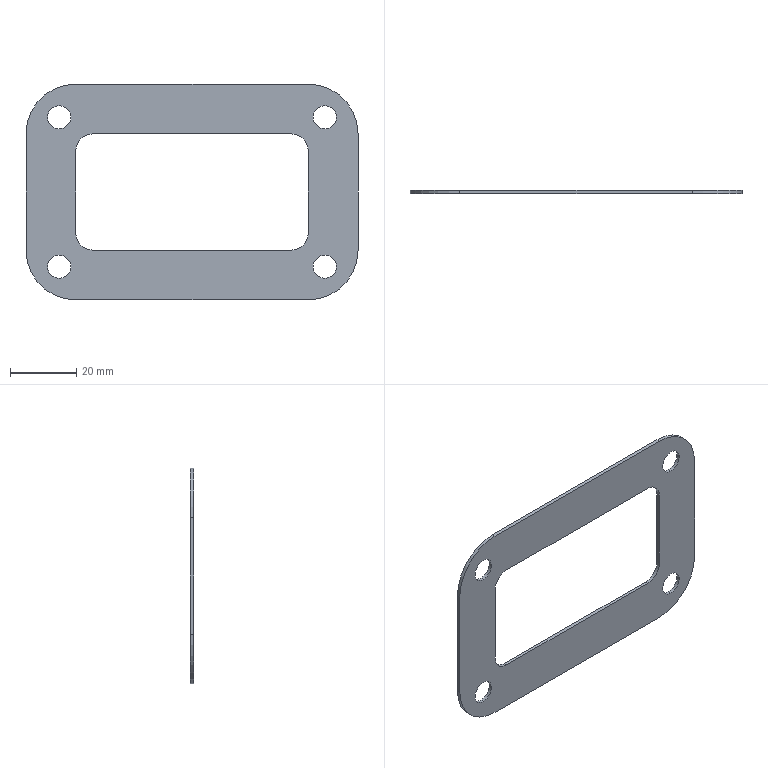Part | SolidWorks | features 3DProfileFeature 1, Extrusion 1, HoleWzd 1, ICE 1, LPattern 1 | 1 solid | 26 faces | box 100 x 1 x 65 mm | volume 3724 mm3 | cylinder 16 | plane 10 | commonest cylinder face diameters 7 x8 10 x4 30 x4
STEP:
#1=CARTESIAN_POINT('',(40.,0.,26.));
#2=VERTEX_POINT('',#1);
#3=CARTESIAN_POINT('',(40.,0.,19.));
#4=VERTEX_POINT('',#3);
#5=CARTESIAN_POINT('',(40.,0.,22.5));
#6=DIRECTION('',(0.,-1.,0.));
#7=DIRECTION('',(0.,0.,-1.));
#8=AXIS2_PLACEMENT_3D('',#5,#6,#7);
#9=CIRCLE('',#8,3.5);
#10=EDGE_CURVE('',#2,#4,#9,.T.);
#11=ORIENTED_EDGE('',*,*,#10,.T.);
#12=CARTESIAN_POINT('',(40.,1.,19.));
#13=VERTEX_POINT('',#12);
#14=CARTESIAN_POINT('',(40.,1.,19.));
#15=DIRECTION('',(0.,1.,0.));
#16=VECTOR('',#15,1000.);
#17=LINE('',#14,#16);
#18=EDGE_CURVE('',#4,#13,#17,.T.);
#19=ORIENTED_EDGE('',*,*,#18,.T.);
#20=CARTESIAN_POINT('',(40.,1.,26.));
#21=VERTEX_POINT('',#20);
#22=CARTESIAN_POINT('',(40.,1.,22.5));
#23=DIRECTION('',(0.,1.,0.));
#24=DIRECTION('',(0.,0.,1.));
#25=AXIS2_PLACEMENT_3D('',#22,#23,#24);
#26=CIRCLE('',#25,3.5);
#27=EDGE_CURVE('',#13,#21,#26,.T.);
#28=ORIENTED_EDGE('',*,*,#27,.T.);
#29=CARTESIAN_POINT('',(40.,1.,26.));
#30=DIRECTION('',(0.,1.,0.));
#31=VECTOR('',#30,1000.);
#32=LINE('',#29,#31);
#33=EDGE_CURVE('',#2,#21,#32,.T.);
#34=ORIENTED_EDGE('',*,*,#33,.F.);
#35=EDGE_LOOP('',(#11,#19,#28,#34));
#36=FACE_OUTER_BOUND('',#35,.T.);
#37=CARTESIAN_POINT('',(40.,1.,22.5));
#38=DIRECTION('',(0.,1.,0.));
#39=DIRECTION('',(0.,0.,1.));
#40=AXIS2_PLACEMENT_3D('',#37,#38,#39);
#41=CYLINDRICAL_SURFACE('',#40,3.5);
#42=ADVANCED_FACE('',(#36),#41,.F.);
#43=CARTESIAN_POINT('',(40.,0.,-19.));
#44=VERTEX_POINT('',#43);
#45=CARTESIAN_POINT('',(40.,0.,-26.));
#46=VERTEX_POINT('',#45);
#47=CARTESIAN_POINT('',(40.,0.,-22.5));
#48=DIRECTION('',(0.,-1.,0.));
#49=DIRECTION('',(0.,0.,-1.));
#50=AXIS2_PLACEMENT_3D('',#47,#48,#49);
#51=CIRCLE('',#50,3.5);
#52=EDGE_CURVE('',#44,#46,#51,.T.);
#53=ORIENTED_EDGE('',*,*,#52,.T.);
#54=CARTESIAN_POINT('',(40.,1.,-26.));
#55=VERTEX_POINT('',#54);
#56=CARTESIAN_POINT('',(40.,1.,-26.));
#57=DIRECTION('',(0.,1.,0.));
#58=VECTOR('',#57,1000.);
#59=LINE('',#56,#58);
#60=EDGE_CURVE('',#46,#55,#59,.T.);
#61=ORIENTED_EDGE('',*,*,#60,.T.);
#62=CARTESIAN_POINT('',(40.,1.,-19.));
#63=VERTEX_POINT('',#62);
#64=CARTESIAN_POINT('',(40.,1.,-22.5));
#65=DIRECTION('',(0.,1.,0.));
#66=DIRECTION('',(0.,0.,1.));
#67=AXIS2_PLACEMENT_3D('',#64,#65,#66);
#68=CIRCLE('',#67,3.5);
#69=EDGE_CURVE('',#55,#63,#68,.T.);
#70=ORIENTED_EDGE('',*,*,#69,.T.);
#71=CARTESIAN_POINT('',(40.,1.,-19.));
#72=DIRECTION('',(0.,1.,0.));
#73=VECTOR('',#72,1000.);
#74=LINE('',#71,#73);
#75=EDGE_CURVE('',#44,#63,#74,.T.);
#76=ORIENTED_EDGE('',*,*,#75,.F.);
#77=EDGE_LOOP('',(#53,#61,#70,#76));
#78=FACE_OUTER_BOUND('',#77,.T.);
#79=CARTESIAN_POINT('',(40.,1.,-22.5));
#80=DIRECTION('',(0.,1.,0.));
#81=DIRECTION('',(0.,0.,1.));
#82=AXIS2_PLACEMENT_3D('',#79,#80,#81);
#83=CYLINDRICAL_SURFACE('',#82,3.5);
#84=ADVANCED_FACE('',(#78),#83,.F.);
#85=CARTESIAN_POINT('',(-40.,0.,26.));
#86=VERTEX_POINT('',#85);
#87=CARTESIAN_POINT('',(-40.,0.,19.));
#88=VERTEX_POINT('',#87);
#89=CARTESIAN_POINT('',(-40.,0.,22.5));
#90=DIRECTION('',(0.,-1.,0.));
#91=DIRECTION('',(0.,0.,-1.));
#92=AXIS2_PLACEMENT_3D('',#89,#90,#91);
#93=CIRCLE('',#92,3.5);
#94=EDGE_CURVE('',#86,#88,#93,.T.);
#95=ORIENTED_EDGE('',*,*,#94,.T.);
#96=CARTESIAN_POINT('',(-40.,1.,19.));
#97=VERTEX_POINT('',#96);
#98=CARTESIAN_POINT('',(-40.,1.,19.));
#99=DIRECTION('',(0.,1.,0.));
#100=VECTOR('',#99,1000.);
#101=LINE('',#98,#100);
#102=EDGE_CURVE('',#88,#97,#101,.T.);
#103=ORIENTED_EDGE('',*,*,#102,.T.);
#104=CARTESIAN_POINT('',(-40.,1.,26.));
#105=VERTEX_POINT('',#104);
#106=CARTESIAN_POINT('',(-40.,1.,22.5));
#107=DIRECTION('',(0.,1.,0.));
#108=DIRECTION('',(0.,0.,1.));
#109=AXIS2_PLACEMENT_3D('',#106,#107,#108);
#110=CIRCLE('',#109,3.5);
#111=EDGE_CURVE('',#97,#105,#110,.T.);
#112=ORIENTED_EDGE('',*,*,#111,.T.);
#113=CARTESIAN_POINT('',(-40.,1.,26.));
#114=DIRECTION('',(0.,1.,0.));
#115=VECTOR('',#114,1000.);
#116=LINE('',#113,#115);
#117=EDGE_CURVE('',#86,#105,#116,.T.);
#118=ORIENTED_EDGE('',*,*,#117,.F.);
#119=EDGE_LOOP('',(#95,#103,#112,#118));
#120=FACE_OUTER_BOUND('',#119,.T.);
#121=CARTESIAN_POINT('',(-40.,1.,22.5));
#122=DIRECTION('',(0.,1.,0.));
#123=DIRECTION('',(0.,0.,1.));
#124=AXIS2_PLACEMENT_3D('',#121,#122,#123);
#125=CYLINDRICAL_SURFACE('',#124,3.5);
#126=ADVANCED_FACE('',(#120),#125,.F.);
#127=CARTESIAN_POINT('',(-40.,0.,-19.));
#128=VERTEX_POINT('',#127);
#129=CARTESIAN_POINT('',(-40.,0.,-26.));
#130=VERTEX_POINT('',#129);
#131=CARTESIAN_POINT('',(-40.,0.,-22.5));
#132=DIRECTION('',(0.,-1.,0.));
#133=DIRECTION('',(0.,0.,-1.));
#134=AXIS2_PLACEMENT_3D('',#131,#132,#133);
#135=CIRCLE('',#134,3.5);
#136=EDGE_CURVE('',#128,#130,#135,.T.);
#137=ORIENTED_EDGE('',*,*,#136,.T.);
#138=CARTESIAN_POINT('',(-40.,1.,-26.));
#139=VERTEX_POINT('',#138);
#140=CARTESIAN_POINT('',(-40.,1.,-26.));
#141=DIRECTION('',(0.,1.,0.));
#142=VECTOR('',#141,1000.);
#143=LINE('',#140,#142);
#144=EDGE_CURVE('',#130,#139,#143,.T.);
#145=ORIENTED_EDGE('',*,*,#144,.T.);
#146=CARTESIAN_POINT('',(-40.,1.,-19.));
#147=VERTEX_POINT('',#146);
#148=CARTESIAN_POINT('',(-40.,1.,-22.5));
#149=DIRECTION('',(0.,1.,0.));
#150=DIRECTION('',(0.,0.,1.));
#151=AXIS2_PLACEMENT_3D('',#148,#149,#150);
#152=CIRCLE('',#151,3.5);
#153=EDGE_CURVE('',#139,#147,#152,.T.);
#154=ORIENTED_EDGE('',*,*,#153,.T.);
#155=CARTESIAN_POINT('',(-40.,1.,-19.));
#156=DIRECTION('',(0.,1.,0.));
#157=VECTOR('',#156,1000.);
#158=LINE('',#155,#157);
#159=EDGE_CURVE('',#128,#147,#158,.T.);
#160=ORIENTED_EDGE('',*,*,#159,.F.);
#161=EDGE_LOOP('',(#137,#145,#154,#160));
#162=FACE_OUTER_BOUND('',#161,.T.);
#163=CARTESIAN_POINT('',(-40.,1.,-22.5));
#164=DIRECTION('',(0.,1.,0.));
#165=DIRECTION('',(0.,0.,1.));
#166=AXIS2_PLACEMENT_3D('',#163,#164,#165);
#167=CYLINDRICAL_SURFACE('',#166,3.5);
#168=ADVANCED_FACE('',(#162),#167,.F.);
#169=CARTESIAN_POINT('',(-40.,1.,22.5));
#170=DIRECTION('',(0.,1.,0.));
#171=DIRECTION('',(0.,0.,1.));
#172=AXIS2_PLACEMENT_3D('',#169,#170,#171);
#173=CIRCLE('',#172,3.5);
#174=EDGE_CURVE('',#105,#97,#173,.T.);
#175=ORIENTED_EDGE('',*,*,#174,.F.);
#176=ORIENTED_EDGE('',*,*,#111,.F.);
#177=EDGE_LOOP('',(#175,#176));
#178=FACE_BOUND('',#177,.T.);
#179=CARTESIAN_POINT('',(-40.,1.,-22.5));
#180=DIRECTION('',(0.,1.,0.));
#181=DIRECTION('',(0.,0.,1.));
#182=AXIS2_PLACEMENT_3D('',#179,#180,#181);
#183=CIRCLE('',#182,3.5);
#184=EDGE_CURVE('',#147,#139,#183,.T.);
#185=ORIENTED_EDGE('',*,*,#184,.F.);
#186=ORIENTED_EDGE('',*,*,#153,.F.);
#187=EDGE_LOOP('',(#185,#186));
#188=FACE_BOUND('',#187,.T.);
#189=CARTESIAN_POINT('',(30.,1.,-17.5));
#190=VERTEX_POINT('',#189);
#191=CARTESIAN_POINT('',(-30.,1.,-17.5));
#192=VERTEX_POINT('',#191);
#193=CARTESIAN_POINT('',(-30.,1.,-17.5));
#194=DIRECTION('',(-1.,0.,0.));
#195=VECTOR('',#194,1000.);
#196=LINE('',#193,#195);
#197=EDGE_CURVE('',#190,#192,#196,.T.);
#198=ORIENTED_EDGE('',*,*,#197,.F.);
#199=CARTESIAN_POINT('',(35.,1.,-12.5));
#200=VERTEX_POINT('',#199);
#201=CARTESIAN_POINT('',(30.,1.,-12.5));
#202=DIRECTION('',(0.,1.,0.));
#203=DIRECTION('',(0.,0.,-1.));
#204=AXIS2_PLACEMENT_3D('',#201,#202,#203);
#205=CIRCLE('',#204,5.);
#206=EDGE_CURVE('',#200,#190,#205,.T.);
#207=ORIENTED_EDGE('',*,*,#206,.F.);
#208=CARTESIAN_POINT('',(35.,1.,12.5));
#209=VERTEX_POINT('',#208);
#210=CARTESIAN_POINT('',(35.,1.,-12.5));
#211=DIRECTION('',(0.,0.,-1.));
#212=VECTOR('',#211,1000.);
#213=LINE('',#210,#212);
#214=EDGE_CURVE('',#209,#200,#213,.T.);
#215=ORIENTED_EDGE('',*,*,#214,.F.);
#216=CARTESIAN_POINT('',(30.,1.,17.5));
#217=VERTEX_POINT('',#216);
#218=CARTESIAN_POINT('',(30.,1.,12.5));
#219=DIRECTION('',(0.,1.,0.));
#220=DIRECTION('',(0.,0.,1.));
#221=AXIS2_PLACEMENT_3D('',#218,#219,#220);
#222=CIRCLE('',#221,5.);
#223=EDGE_CURVE('',#217,#209,#222,.T.);
#224=ORIENTED_EDGE('',*,*,#223,.F.);
#225=CARTESIAN_POINT('',(-30.,1.,17.5));
#226=VERTEX_POINT('',#225);
#227=CARTESIAN_POINT('',(-30.,1.,17.5));
#228=DIRECTION('',(1.,0.,0.));
#229=VECTOR('',#228,1000.);
#230=LINE('',#227,#229);
#231=EDGE_CURVE('',#226,#217,#230,.T.);
#232=ORIENTED_EDGE('',*,*,#231,.F.);
#233=CARTESIAN_POINT('',(-35.,1.,12.5));
#234=VERTEX_POINT('',#233);
#235=CARTESIAN_POINT('',(-30.,1.,12.5));
#236=DIRECTION('',(0.,1.,0.));
#237=DIRECTION('',(0.,0.,1.));
#238=AXIS2_PLACEMENT_3D('',#235,#236,#237);
#239=CIRCLE('',#238,5.);
#240=EDGE_CURVE('',#234,#226,#239,.T.);
#241=ORIENTED_EDGE('',*,*,#240,.F.);
#242=CARTESIAN_POINT('',(-35.,1.,-12.5));
#243=VERTEX_POINT('',#242);
#244=CARTESIAN_POINT('',(-35.,1.,-12.5));
#245=DIRECTION('',(0.,0.,1.));
#246=VECTOR('',#245,1000.);
#247=LINE('',#244,#246);
#248=EDGE_CURVE('',#243,#234,#247,.T.);
#249=ORIENTED_EDGE('',*,*,#248,.F.);
#250=CARTESIAN_POINT('',(-30.,1.,-12.5));
#251=DIRECTION('',(0.,1.,0.));
#252=DIRECTION('',(0.,0.,1.));
#253=AXIS2_PLACEMENT_3D('',#250,#251,#252);
#254=CIRCLE('',#253,5.);
#255=EDGE_CURVE('',#192,#243,#254,.T.);
#256=ORIENTED_EDGE('',*,*,#255,.F.);
#257=EDGE_LOOP('',(#198,#207,#215,#224,#232,#241,#249,#256));
#258=FACE_BOUND('',#257,.T.);
#259=CARTESIAN_POINT('',(50.,1.,-17.5));
#260=VERTEX_POINT('',#259);
#261=CARTESIAN_POINT('',(35.,1.,-32.5));
#262=VERTEX_POINT('',#261);
#263=CARTESIAN_POINT('',(35.,1.,-17.5));
#264=DIRECTION('',(0.,1.,0.));
#265=DIRECTION('',(0.,0.,-1.));
#266=AXIS2_PLACEMENT_3D('',#263,#264,#265);
#267=CIRCLE('',#266,15.);
#268=EDGE_CURVE('',#260,#262,#267,.T.);
#269=ORIENTED_EDGE('',*,*,#268,.T.);
#270=CARTESIAN_POINT('',(-35.,1.,-32.5));
#271=VERTEX_POINT('',#270);
#272=CARTESIAN_POINT('',(-35.,1.,-32.5));
#273=DIRECTION('',(-1.,0.,0.));
#274=VECTOR('',#273,1000.);
#275=LINE('',#272,#274);
#276=EDGE_CURVE('',#262,#271,#275,.T.);
#277=ORIENTED_EDGE('',*,*,#276,.T.);
#278=CARTESIAN_POINT('',(-50.,1.,-17.5));
#279=VERTEX_POINT('',#278);
#280=CARTESIAN_POINT('',(-35.,1.,-17.5));
#281=DIRECTION('',(0.,1.,0.));
#282=DIRECTION('',(0.,0.,1.));
#283=AXIS2_PLACEMENT_3D('',#280,#281,#282);
#284=CIRCLE('',#283,15.);
#285=EDGE_CURVE('',#271,#279,#284,.T.);
#286=ORIENTED_EDGE('',*,*,#285,.T.);
#287=CARTESIAN_POINT('',(-50.,1.,17.5));
#288=VERTEX_POINT('',#287);
#289=CARTESIAN_POINT('',(-50.,1.,-17.5));
#290=DIRECTION('',(0.,0.,1.));
#291=VECTOR('',#290,1000.);
#292=LINE('',#289,#291);
#293=EDGE_CURVE('',#279,#288,#292,.T.);
#294=ORIENTED_EDGE('',*,*,#293,.T.);
#295=CARTESIAN_POINT('',(-35.,1.,32.5));
#296=VERTEX_POINT('',#295);
#297=CARTESIAN_POINT('',(-35.,1.,17.5));
#298=DIRECTION('',(0.,1.,0.));
#299=DIRECTION('',(0.,0.,1.));
#300=AXIS2_PLACEMENT_3D('',#297,#298,#299);
#301=CIRCLE('',#300,15.);
#302=EDGE_CURVE('',#288,#296,#301,.T.);
#303=ORIENTED_EDGE('',*,*,#302,.T.);
#304=CARTESIAN_POINT('',(35.,1.,32.5));
#305=VERTEX_POINT('',#304);
#306=CARTESIAN_POINT('',(-35.,1.,32.5));
#307=DIRECTION('',(1.,0.,0.));
#308=VECTOR('',#307,1000.);
#309=LINE('',#306,#308);
#310=EDGE_CURVE('',#296,#305,#309,.T.);
#311=ORIENTED_EDGE('',*,*,#310,.T.);
#312=CARTESIAN_POINT('',(50.,1.,17.5));
#313=VERTEX_POINT('',#312);
#314=CARTESIAN_POINT('',(35.,1.,17.5));
#315=DIRECTION('',(0.,1.,0.));
#316=DIRECTION('',(0.,0.,1.));
#317=AXIS2_PLACEMENT_3D('',#314,#315,#316);
#318=CIRCLE('',#317,15.);
#319=EDGE_CURVE('',#305,#313,#318,.T.);
#320=ORIENTED_EDGE('',*,*,#319,.T.);
#321=CARTESIAN_POINT('',(50.,1.,-17.5));
#322=DIRECTION('',(0.,0.,-1.));
#323=VECTOR('',#322,1000.);
#324=LINE('',#321,#323);
#325=EDGE_CURVE('',#313,#260,#324,.T.);
#326=ORIENTED_EDGE('',*,*,#325,.T.);
#327=EDGE_LOOP('',(#269,#277,#286,#294,#303,#311,#320,#326));
#328=FACE_OUTER_BOUND('',#327,.T.);
#329=CARTESIAN_POINT('',(40.,1.,-22.5));
#330=DIRECTION('',(0.,1.,0.));
#331=DIRECTION('',(0.,0.,1.));
#332=AXIS2_PLACEMENT_3D('',#329,#330,#331);
#333=CIRCLE('',#332,3.5);
#334=EDGE_CURVE('',#63,#55,#333,.T.);
#335=ORIENTED_EDGE('',*,*,#334,.F.);
#336=ORIENTED_EDGE('',*,*,#69,.F.);
#337=EDGE_LOOP('',(#335,#336));
#338=FACE_BOUND('',#337,.T.);
#339=CARTESIAN_POINT('',(40.,1.,22.5));
#340=DIRECTION('',(0.,1.,0.));
#341=DIRECTION('',(0.,0.,1.));
#342=AXIS2_PLACEMENT_3D('',#339,#340,#341);
#343=CIRCLE('',#342,3.5);
#344=EDGE_CURVE('',#21,#13,#343,.T.);
#345=ORIENTED_EDGE('',*,*,#344,.F.);
#346=ORIENTED_EDGE('',*,*,#27,.F.);
#347=EDGE_LOOP('',(#345,#346));
#348=FACE_BOUND('',#347,.T.);
#349=CARTESIAN_POINT('',(35.,1.,-17.5));
#350=DIRECTION('',(0.,-1.,0.));
#351=DIRECTION('',(0.,0.,-1.));
#352=AXIS2_PLACEMENT_3D('',#349,#350,#351);
#353=PLANE('',#352);
#354=ADVANCED_FACE('',(#178,#188,#258,#328,#338,#348),#353,.F.);
#355=CARTESIAN_POINT('',(50.,0.,-17.5));
#356=VERTEX_POINT('',#355);
#357=CARTESIAN_POINT('',(35.,0.,-32.5));
#358=VERTEX_POINT('',#357);
#359=CARTESIAN_POINT('',(35.,0.,-17.5));
#360=DIRECTION('',(0.,1.,0.));
#361=DIRECTION('',(0.,0.,-1.));
#362=AXIS2_PLACEMENT_3D('',#359,#360,#361);
#363=CIRCLE('',#362,15.);
#364=EDGE_CURVE('',#356,#358,#363,.T.);
#365=ORIENTED_EDGE('',*,*,#364,.T.);
#366=CARTESIAN_POINT('',(35.,1.,-32.5));
#367=DIRECTION('',(0.,-1.,0.));
#368=VECTOR('',#367,1000.);
#369=LINE('',#366,#368);
#370=EDGE_CURVE('',#262,#358,#369,.T.);
#371=ORIENTED_EDGE('',*,*,#370,.F.);
#372=ORIENTED_EDGE('',*,*,#268,.F.);
#373=CARTESIAN_POINT('',(50.,1.,-17.5));
#374=DIRECTION('',(0.,-1.,0.));
#375=VECTOR('',#374,1000.);
#376=LINE('',#373,#375);
#377=EDGE_CURVE('',#260,#356,#376,.T.);
#378=ORIENTED_EDGE('',*,*,#377,.T.);
#379=EDGE_LOOP('',(#365,#371,#372,#378));
#380=FACE_OUTER_BOUND('',#379,.T.);
#381=CARTESIAN_POINT('',(35.,1.,-17.5));
#382=DIRECTION('',(0.,-1.,0.));
#383=DIRECTION('',(0.,0.,-1.));
#384=AXIS2_PLACEMENT_3D('',#381,#382,#383);
#385=CYLINDRICAL_SURFACE('',#384,15.);
#386=ADVANCED_FACE('',(#380),#385,.T.);
#387=CARTESIAN_POINT('',(-35.,0.,-32.5));
#388=VERTEX_POINT('',#387);
#389=CARTESIAN_POINT('',(-35.,0.,-32.5));
#390=DIRECTION('',(-1.,0.,0.));
#391=VECTOR('',#390,1000.);
#392=LINE('',#389,#391);
#393=EDGE_CURVE('',#358,#388,#392,.T.);
#394=ORIENTED_EDGE('',*,*,#393,.T.);
#395=CARTESIAN_POINT('',(-35.,1.,-32.5));
#396=DIRECTION('',(0.,-1.,0.));
#397=VECTOR('',#396,1000.);
#398=LINE('',#395,#397);
#399=EDGE_CURVE('',#271,#388,#398,.T.);
#400=ORIENTED_EDGE('',*,*,#399,.F.);
#401=ORIENTED_EDGE('',*,*,#276,.F.);
#402=ORIENTED_EDGE('',*,*,#370,.T.);
#403=EDGE_LOOP('',(#394,#400,#401,#402));
#404=FACE_OUTER_BOUND('',#403,.T.);
#405=CARTESIAN_POINT('',(-35.,1.,-32.5));
#406=DIRECTION('',(0.,0.,1.));
#407=DIRECTION('',(1.,0.,0.));
#408=AXIS2_PLACEMENT_3D('',#405,#406,#407);
#409=PLANE('',#408);
#410=ADVANCED_FACE('',(#404),#409,.F.);
#411=CARTESIAN_POINT('',(-50.,0.,-17.5));
#412=VERTEX_POINT('',#411);
#413=CARTESIAN_POINT('',(-35.,0.,-17.5));
#414=DIRECTION('',(0.,1.,0.));
#415=DIRECTION('',(0.,0.,1.));
#416=AXIS2_PLACEMENT_3D('',#413,#414,#415);
#417=CIRCLE('',#416,15.);
#418=EDGE_CURVE('',#388,#412,#417,.T.);
#419=ORIENTED_EDGE('',*,*,#418,.T.);
#420=CARTESIAN_POINT('',(-50.,1.,-17.5));
#421=DIRECTION('',(0.,-1.,0.));
#422=VECTOR('',#421,1000.);
#423=LINE('',#420,#422);
#424=EDGE_CURVE('',#279,#412,#423,.T.);
#425=ORIENTED_EDGE('',*,*,#424,.F.);
#426=ORIENTED_EDGE('',*,*,#285,.F.);
#427=ORIENTED_EDGE('',*,*,#399,.T.);
#428=EDGE_LOOP('',(#419,#425,#426,#427));
#429=FACE_OUTER_BOUND('',#428,.T.);
#430=CARTESIAN_POINT('',(-35.,1.,-17.5));
#431=DIRECTION('',(0.,-1.,0.));
#432=DIRECTION('',(0.,0.,-1.));
#433=AXIS2_PLACEMENT_3D('',#430,#431,#432);
#434=CYLINDRICAL_SURFACE('',#433,15.);
#435=ADVANCED_FACE('',(#429),#434,.T.);
#436=CARTESIAN_POINT('',(-50.,0.,17.5));
#437=VERTEX_POINT('',#436);
#438=CARTESIAN_POINT('',(-50.,0.,-17.5));
#439=DIRECTION('',(0.,0.,1.));
#440=VECTOR('',#439,1000.);
#441=LINE('',#438,#440);
#442=EDGE_CURVE('',#412,#437,#441,.T.);
#443=ORIENTED_EDGE('',*,*,#442,.T.);
#444=CARTESIAN_POINT('',(-50.,1.,17.5));
#445=DIRECTION('',(0.,-1.,0.));
#446=VECTOR('',#445,1000.);
#447=LINE('',#444,#446);
#448=EDGE_CURVE('',#288,#437,#447,.T.);
#449=ORIENTED_EDGE('',*,*,#448,.F.);
#450=ORIENTED_EDGE('',*,*,#293,.F.);
#451=ORIENTED_EDGE('',*,*,#424,.T.);
#452=EDGE_LOOP('',(#443,#449,#450,#451));
#453=FACE_OUTER_BOUND('',#452,.T.);
#454=CARTESIAN_POINT('',(-50.,1.,-17.5));
#455=DIRECTION('',(1.,0.,0.));
#456=DIRECTION('',(0.,0.,-1.));
#457=AXIS2_PLACEMENT_3D('',#454,#455,#456);
#458=PLANE('',#457);
#459=ADVANCED_FACE('',(#453),#458,.F.);
#460=CARTESIAN_POINT('',(-35.,0.,32.5));
#461=VERTEX_POINT('',#460);
#462=CARTESIAN_POINT('',(-35.,0.,17.5));
#463=DIRECTION('',(0.,1.,0.));
#464=DIRECTION('',(0.,0.,1.));
#465=AXIS2_PLACEMENT_3D('',#462,#463,#464);
#466=CIRCLE('',#465,15.);
#467=EDGE_CURVE('',#437,#461,#466,.T.);
#468=ORIENTED_EDGE('',*,*,#467,.T.);
#469=CARTESIAN_POINT('',(-35.,1.,32.5));
#470=DIRECTION('',(0.,-1.,0.));
#471=VECTOR('',#470,1000.);
#472=LINE('',#469,#471);
#473=EDGE_CURVE('',#296,#461,#472,.T.);
#474=ORIENTED_EDGE('',*,*,#473,.F.);
#475=ORIENTED_EDGE('',*,*,#302,.F.);
#476=ORIENTED_EDGE('',*,*,#448,.T.);
#477=EDGE_LOOP('',(#468,#474,#475,#476));
#478=FACE_OUTER_BOUND('',#477,.T.);
#479=CARTESIAN_POINT('',(-35.,1.,17.5));
#480=DIRECTION('',(0.,-1.,0.));
#481=DIRECTION('',(0.,0.,-1.));
#482=AXIS2_PLACEMENT_3D('',#479,#480,#481);
#483=CYLINDRICAL_SURFACE('',#482,15.);
#484=ADVANCED_FACE('',(#478),#483,.T.);
#485=CARTESIAN_POINT('',(35.,0.,32.5));
#486=VERTEX_POINT('',#485);
#487=CARTESIAN_POINT('',(-35.,0.,32.5));
#488=DIRECTION('',(1.,0.,0.));
#489=VECTOR('',#488,1000.);
#490=LINE('',#487,#489);
#491=EDGE_CURVE('',#461,#486,#490,.T.);
#492=ORIENTED_EDGE('',*,*,#491,.T.);
#493=CARTESIAN_POINT('',(35.,1.,32.5));
#494=DIRECTION('',(0.,-1.,0.));
#495=VECTOR('',#494,1000.);
#496=LINE('',#493,#495);
#497=EDGE_CURVE('',#305,#486,#496,.T.);
#498=ORIENTED_EDGE('',*,*,#497,.F.);
#499=ORIENTED_EDGE('',*,*,#310,.F.);
#500=ORIENTED_EDGE('',*,*,#473,.T.);
#501=EDGE_LOOP('',(#492,#498,#499,#500));
#502=FACE_OUTER_BOUND('',#501,.T.);
#503=CARTESIAN_POINT('',(-35.,1.,32.5));
#504=DIRECTION('',(0.,0.,-1.));
#505=DIRECTION('',(-1.,0.,0.));
#506=AXIS2_PLACEMENT_3D('',#503,#504,#505);
#507=PLANE('',#506);
#508=ADVANCED_FACE('',(#502),#507,.F.);
#509=CARTESIAN_POINT('',(50.,0.,17.5));
#510=VERTEX_POINT('',#509);
#511=CARTESIAN_POINT('',(35.,0.,17.5));
#512=DIRECTION('',(0.,1.,0.));
#513=DIRECTION('',(0.,0.,1.));
#514=AXIS2_PLACEMENT_3D('',#511,#512,#513);
#515=CIRCLE('',#514,15.);
#516=EDGE_CURVE('',#486,#510,#515,.T.);
#517=ORIENTED_EDGE('',*,*,#516,.T.);
#518=CARTESIAN_POINT('',(50.,1.,17.5));
#519=DIRECTION('',(0.,-1.,0.));
#520=VECTOR('',#519,1000.);
#521=LINE('',#518,#520);
#522=EDGE_CURVE('',#313,#510,#521,.T.);
#523=ORIENTED_EDGE('',*,*,#522,.F.);
#524=ORIENTED_EDGE('',*,*,#319,.F.);
#525=ORIENTED_EDGE('',*,*,#497,.T.);
#526=EDGE_LOOP('',(#517,#523,#524,#525));
#527=FACE_OUTER_BOUND('',#526,.T.);
#528=CARTESIAN_POINT('',(35.,1.,17.5));
#529=DIRECTION('',(0.,-1.,0.));
#530=DIRECTION('',(0.,0.,-1.));
#531=AXIS2_PLACEMENT_3D('',#528,#529,#530);
#532=CYLINDRICAL_SURFACE('',#531,15.);
#533=ADVANCED_FACE('',(#527),#532,.T.);
#534=CARTESIAN_POINT('',(50.,0.,-17.5));
#535=DIRECTION('',(0.,0.,-1.));
#536=VECTOR('',#535,1000.);
#537=LINE('',#534,#536);
#538=EDGE_CURVE('',#510,#356,#537,.T.);
#539=ORIENTED_EDGE('',*,*,#538,.T.);
#540=ORIENTED_EDGE('',*,*,#377,.F.);
#541=ORIENTED_EDGE('',*,*,#325,.F.);
#542=ORIENTED_EDGE('',*,*,#522,.T.);
#543=EDGE_LOOP('',(#539,#540,#541,#542));
#544=FACE_OUTER_BOUND('',#543,.T.);
#545=CARTESIAN_POINT('',(50.,1.,-17.5));
#546=DIRECTION('',(-1.,0.,0.));
#547=DIRECTION('',(0.,0.,1.));
#548=AXIS2_PLACEMENT_3D('',#545,#546,#547);
#549=PLANE('',#548);
#550=ADVANCED_FACE('',(#544),#549,.F.);
#551=ORIENTED_EDGE('',*,*,#10,.F.);
#552=CARTESIAN_POINT('',(40.,0.,22.5));
#553=DIRECTION('',(0.,-1.,0.));
#554=DIRECTION('',(0.,0.,-1.));
#555=AXIS2_PLACEMENT_3D('',#552,#553,#554);
#556=CIRCLE('',#555,3.5);
#557=EDGE_CURVE('',#4,#2,#556,.T.);
#558=ORIENTED_EDGE('',*,*,#557,.F.);
#559=EDGE_LOOP('',(#551,#558));
#560=FACE_BOUND('',#559,.T.);
#561=ORIENTED_EDGE('',*,*,#52,.F.);
#562=CARTESIAN_POINT('',(40.,0.,-22.5));
#563=DIRECTION('',(0.,-1.,0.));
#564=DIRECTION('',(0.,0.,-1.));
#565=AXIS2_PLACEMENT_3D('',#562,#563,#564);
#566=CIRCLE('',#565,3.5);
#567=EDGE_CURVE('',#46,#44,#566,.T.);
#568=ORIENTED_EDGE('',*,*,#567,.F.);
#569=EDGE_LOOP('',(#561,#568));
#570=FACE_BOUND('',#569,.T.);
#571=ORIENTED_EDGE('',*,*,#94,.F.);
#572=CARTESIAN_POINT('',(-40.,0.,22.5));
#573=DIRECTION('',(0.,-1.,0.));
#574=DIRECTION('',(0.,0.,-1.));
#575=AXIS2_PLACEMENT_3D('',#572,#573,#574);
#576=CIRCLE('',#575,3.5);
#577=EDGE_CURVE('',#88,#86,#576,.T.);
#578=ORIENTED_EDGE('',*,*,#577,.F.);
#579=EDGE_LOOP('',(#571,#578));
#580=FACE_BOUND('',#579,.T.);
#581=ORIENTED_EDGE('',*,*,#136,.F.);
#582=CARTESIAN_POINT('',(-40.,0.,-22.5));
#583=DIRECTION('',(0.,-1.,0.));
#584=DIRECTION('',(0.,0.,-1.));
#585=AXIS2_PLACEMENT_3D('',#582,#583,#584);
#586=CIRCLE('',#585,3.5);
#587=EDGE_CURVE('',#130,#128,#586,.T.);
#588=ORIENTED_EDGE('',*,*,#587,.F.);
#589=EDGE_LOOP('',(#581,#588));
#590=FACE_BOUND('',#589,.T.);
#591=CARTESIAN_POINT('',(35.,0.,-12.5));
#592=VERTEX_POINT('',#591);
#593=CARTESIAN_POINT('',(30.,0.,-17.5));
#594=VERTEX_POINT('',#593);
#595=CARTESIAN_POINT('',(30.,0.,-12.5));
#596=DIRECTION('',(0.,1.,0.));
#597=DIRECTION('',(0.,0.,-1.));
#598=AXIS2_PLACEMENT_3D('',#595,#596,#597);
#599=CIRCLE('',#598,5.);
#600=EDGE_CURVE('',#592,#594,#599,.T.);
#601=ORIENTED_EDGE('',*,*,#600,.T.);
#602=CARTESIAN_POINT('',(-30.,0.,-17.5));
#603=VERTEX_POINT('',#602);
#604=CARTESIAN_POINT('',(-30.,0.,-17.5));
#605=DIRECTION('',(-1.,0.,0.));
#606=VECTOR('',#605,1000.);
#607=LINE('',#604,#606);
#608=EDGE_CURVE('',#594,#603,#607,.T.);
#609=ORIENTED_EDGE('',*,*,#608,.T.);
#610=CARTESIAN_POINT('',(-35.,0.,-12.5));
#611=VERTEX_POINT('',#610);
#612=CARTESIAN_POINT('',(-30.,0.,-12.5));
#613=DIRECTION('',(0.,1.,0.));
#614=DIRECTION('',(0.,0.,1.));
#615=AXIS2_PLACEMENT_3D('',#612,#613,#614);
#616=CIRCLE('',#615,5.);
#617=EDGE_CURVE('',#603,#611,#616,.T.);
#618=ORIENTED_EDGE('',*,*,#617,.T.);
#619=CARTESIAN_POINT('',(-35.,0.,12.5));
#620=VERTEX_POINT('',#619);
#621=CARTESIAN_POINT('',(-35.,0.,-12.5));
#622=DIRECTION('',(0.,0.,1.));
#623=VECTOR('',#622,1000.);
#624=LINE('',#621,#623);
#625=EDGE_CURVE('',#611,#620,#624,.T.);
#626=ORIENTED_EDGE('',*,*,#625,.T.);
#627=CARTESIAN_POINT('',(-30.,0.,17.5));
#628=VERTEX_POINT('',#627);
#629=CARTESIAN_POINT('',(-30.,0.,12.5));
#630=DIRECTION('',(0.,1.,0.));
#631=DIRECTION('',(0.,0.,1.));
#632=AXIS2_PLACEMENT_3D('',#629,#630,#631);
#633=CIRCLE('',#632,5.);
#634=EDGE_CURVE('',#620,#628,#633,.T.);
#635=ORIENTED_EDGE('',*,*,#634,.T.);
#636=CARTESIAN_POINT('',(30.,0.,17.5));
#637=VERTEX_POINT('',#636);
#638=CARTESIAN_POINT('',(-30.,0.,17.5));
#639=DIRECTION('',(1.,0.,0.));
#640=VECTOR('',#639,1000.);
#641=LINE('',#638,#640);
#642=EDGE_CURVE('',#628,#637,#641,.T.);
#643=ORIENTED_EDGE('',*,*,#642,.T.);
#644=CARTESIAN_POINT('',(35.,0.,12.5));
#645=VERTEX_POINT('',#644);
#646=CARTESIAN_POINT('',(30.,0.,12.5));
#647=DIRECTION('',(0.,1.,0.));
#648=DIRECTION('',(0.,0.,1.));
#649=AXIS2_PLACEMENT_3D('',#646,#647,#648);
#650=CIRCLE('',#649,5.);
#651=EDGE_CURVE('',#637,#645,#650,.T.);
#652=ORIENTED_EDGE('',*,*,#651,.T.);
#653=CARTESIAN_POINT('',(35.,0.,-12.5));
#654=DIRECTION('',(0.,0.,-1.));
#655=VECTOR('',#654,1000.);
#656=LINE('',#653,#655);
#657=EDGE_CURVE('',#645,#592,#656,.T.);
#658=ORIENTED_EDGE('',*,*,#657,.T.);
#659=EDGE_LOOP('',(#601,#609,#618,#626,#635,#643,#652,#658));
#660=FACE_BOUND('',#659,.T.);
#661=ORIENTED_EDGE('',*,*,#364,.F.);
#662=ORIENTED_EDGE('',*,*,#538,.F.);
#663=ORIENTED_EDGE('',*,*,#516,.F.);
#664=ORIENTED_EDGE('',*,*,#491,.F.);
#665=ORIENTED_EDGE('',*,*,#467,.F.);
#666=ORIENTED_EDGE('',*,*,#442,.F.);
#667=ORIENTED_EDGE('',*,*,#418,.F.);
#668=ORIENTED_EDGE('',*,*,#393,.F.);
#669=EDGE_LOOP('',(#661,#662,#663,#664,#665,#666,#667,#668));
#670=FACE_OUTER_BOUND('',#669,.T.);
#671=CARTESIAN_POINT('',(35.,0.,-17.5));
#672=DIRECTION('',(0.,-1.,0.));
#673=DIRECTION('',(0.,0.,-1.));
#674=AXIS2_PLACEMENT_3D('',#671,#672,#673);
#675=PLANE('',#674);
#676=ADVANCED_FACE('',(#560,#570,#580,#590,#660,#670),#675,.T.);
#677=ORIENTED_EDGE('',*,*,#206,.T.);
#678=CARTESIAN_POINT('',(30.,0.,-17.5));
#679=DIRECTION('',(0.,1.,0.));
#680=VECTOR('',#679,1000.);
#681=LINE('',#678,#680);
#682=EDGE_CURVE('',#594,#190,#681,.T.);
#683=ORIENTED_EDGE('',*,*,#682,.F.);
#684=ORIENTED_EDGE('',*,*,#600,.F.);
#685=CARTESIAN_POINT('',(35.,0.,-12.5));
#686=DIRECTION('',(0.,1.,0.));
#687=VECTOR('',#686,1000.);
#688=LINE('',#685,#687);
#689=EDGE_CURVE('',#592,#200,#688,.T.);
#690=ORIENTED_EDGE('',*,*,#689,.T.);
#691=EDGE_LOOP('',(#677,#683,#684,#690));
#692=FACE_OUTER_BOUND('',#691,.T.);
#693=CARTESIAN_POINT('',(30.,0.,-12.5));
#694=DIRECTION('',(0.,1.,0.));
#695=DIRECTION('',(0.,0.,1.));
#696=AXIS2_PLACEMENT_3D('',#693,#694,#695);
#697=CYLINDRICAL_SURFACE('',#696,5.);
#698=ADVANCED_FACE('',(#692),#697,.F.);
#699=ORIENTED_EDGE('',*,*,#214,.T.);
#700=ORIENTED_EDGE('',*,*,#689,.F.);
#701=ORIENTED_EDGE('',*,*,#657,.F.);
#702=CARTESIAN_POINT('',(35.,0.,12.5));
#703=DIRECTION('',(0.,1.,0.));
#704=VECTOR('',#703,1000.);
#705=LINE('',#702,#704);
#706=EDGE_CURVE('',#645,#209,#705,.T.);
#707=ORIENTED_EDGE('',*,*,#706,.T.);
#708=EDGE_LOOP('',(#699,#700,#701,#707));
#709=FACE_OUTER_BOUND('',#708,.T.);
#710=CARTESIAN_POINT('',(35.,0.,-12.5));
#711=DIRECTION('',(1.,0.,0.));
#712=DIRECTION('',(0.,0.,-1.));
#713=AXIS2_PLACEMENT_3D('',#710,#711,#712);
#714=PLANE('',#713);
#715=ADVANCED_FACE('',(#709),#714,.F.);
#716=ORIENTED_EDGE('',*,*,#223,.T.);
#717=ORIENTED_EDGE('',*,*,#706,.F.);
#718=ORIENTED_EDGE('',*,*,#651,.F.);
#719=CARTESIAN_POINT('',(30.,0.,17.5));
#720=DIRECTION('',(0.,1.,0.));
#721=VECTOR('',#720,1000.);
#722=LINE('',#719,#721);
#723=EDGE_CURVE('',#637,#217,#722,.T.);
#724=ORIENTED_EDGE('',*,*,#723,.T.);
#725=EDGE_LOOP('',(#716,#717,#718,#724));
#726=FACE_OUTER_BOUND('',#725,.T.);
#727=CARTESIAN_POINT('',(30.,0.,12.5));
#728=DIRECTION('',(0.,1.,0.));
#729=DIRECTION('',(0.,0.,1.));
#730=AXIS2_PLACEMENT_3D('',#727,#728,#729);
#731=CYLINDRICAL_SURFACE('',#730,5.);
#732=ADVANCED_FACE('',(#726),#731,.F.);
#733=ORIENTED_EDGE('',*,*,#231,.T.);
#734=ORIENTED_EDGE('',*,*,#723,.F.);
#735=ORIENTED_EDGE('',*,*,#642,.F.);
#736=CARTESIAN_POINT('',(-30.,0.,17.5));
#737=DIRECTION('',(0.,1.,0.));
#738=VECTOR('',#737,1000.);
#739=LINE('',#736,#738);
#740=EDGE_CURVE('',#628,#226,#739,.T.);
#741=ORIENTED_EDGE('',*,*,#740,.T.);
#742=EDGE_LOOP('',(#733,#734,#735,#741));
#743=FACE_OUTER_BOUND('',#742,.T.);
#744=CARTESIAN_POINT('',(-30.,0.,17.5));
#745=DIRECTION('',(0.,0.,1.));
#746=DIRECTION('',(1.,0.,0.));
#747=AXIS2_PLACEMENT_3D('',#744,#745,#746);
#748=PLANE('',#747);
#749=ADVANCED_FACE('',(#743),#748,.F.);
#750=ORIENTED_EDGE('',*,*,#240,.T.);
#751=ORIENTED_EDGE('',*,*,#740,.F.);
#752=ORIENTED_EDGE('',*,*,#634,.F.);
#753=CARTESIAN_POINT('',(-35.,0.,12.5));
#754=DIRECTION('',(0.,1.,0.));
#755=VECTOR('',#754,1000.);
#756=LINE('',#753,#755);
#757=EDGE_CURVE('',#620,#234,#756,.T.);
#758=ORIENTED_EDGE('',*,*,#757,.T.);
#759=EDGE_LOOP('',(#750,#751,#752,#758));
#760=FACE_OUTER_BOUND('',#759,.T.);
#761=CARTESIAN_POINT('',(-30.,0.,12.5));
#762=DIRECTION('',(0.,1.,0.));
#763=DIRECTION('',(0.,0.,1.));
#764=AXIS2_PLACEMENT_3D('',#761,#762,#763);
#765=CYLINDRICAL_SURFACE('',#764,5.);
#766=ADVANCED_FACE('',(#760),#765,.F.);
#767=ORIENTED_EDGE('',*,*,#248,.T.);
#768=ORIENTED_EDGE('',*,*,#757,.F.);
#769=ORIENTED_EDGE('',*,*,#625,.F.);
#770=CARTESIAN_POINT('',(-35.,0.,-12.5));
#771=DIRECTION('',(0.,1.,0.));
#772=VECTOR('',#771,1000.);
#773=LINE('',#770,#772);
#774=EDGE_CURVE('',#611,#243,#773,.T.);
#775=ORIENTED_EDGE('',*,*,#774,.T.);
#776=EDGE_LOOP('',(#767,#768,#769,#775));
#777=FACE_OUTER_BOUND('',#776,.T.);
#778=CARTESIAN_POINT('',(-35.,0.,-12.5));
#779=DIRECTION('',(-1.,0.,0.));
#780=DIRECTION('',(0.,0.,1.));
#781=AXIS2_PLACEMENT_3D('',#778,#779,#780);
#782=PLANE('',#781);
#783=ADVANCED_FACE('',(#777),#782,.F.);
#784=ORIENTED_EDGE('',*,*,#255,.T.);
#785=ORIENTED_EDGE('',*,*,#774,.F.);
#786=ORIENTED_EDGE('',*,*,#617,.F.);
#787=CARTESIAN_POINT('',(-30.,0.,-17.5));
#788=DIRECTION('',(0.,1.,0.));
#789=VECTOR('',#788,1000.);
#790=LINE('',#787,#789);
#791=EDGE_CURVE('',#603,#192,#790,.T.);
#792=ORIENTED_EDGE('',*,*,#791,.T.);
#793=EDGE_LOOP('',(#784,#785,#786,#792));
#794=FACE_OUTER_BOUND('',#793,.T.);
#795=CARTESIAN_POINT('',(-30.,0.,-12.5));
#796=DIRECTION('',(0.,1.,0.));
#797=DIRECTION('',(0.,0.,1.));
#798=AXIS2_PLACEMENT_3D('',#795,#796,#797);
#799=CYLINDRICAL_SURFACE('',#798,5.);
#800=ADVANCED_FACE('',(#794),#799,.F.);
#801=ORIENTED_EDGE('',*,*,#197,.T.);
#802=ORIENTED_EDGE('',*,*,#791,.F.);
#803=ORIENTED_EDGE('',*,*,#608,.F.);
#804=ORIENTED_EDGE('',*,*,#682,.T.);
#805=EDGE_LOOP('',(#801,#802,#803,#804));
#806=FACE_OUTER_BOUND('',#805,.T.);
#807=CARTESIAN_POINT('',(-30.,0.,-17.5));
#808=DIRECTION('',(0.,0.,-1.));
#809=DIRECTION('',(-1.,0.,0.));
#810=AXIS2_PLACEMENT_3D('',#807,#808,#809);
#811=PLANE('',#810);
#812=ADVANCED_FACE('',(#806),#811,.F.);
#813=ORIENTED_EDGE('',*,*,#144,.F.);
#814=ORIENTED_EDGE('',*,*,#587,.T.);
#815=ORIENTED_EDGE('',*,*,#159,.T.);
#816=ORIENTED_EDGE('',*,*,#184,.T.);
#817=EDGE_LOOP('',(#813,#814,#815,#816));
#818=FACE_OUTER_BOUND('',#817,.T.);
#819=CARTESIAN_POINT('',(-40.,1.,-22.5));
#820=DIRECTION('',(0.,1.,0.));
#821=DIRECTION('',(0.,0.,1.));
#822=AXIS2_PLACEMENT_3D('',#819,#820,#821);
#823=CYLINDRICAL_SURFACE('',#822,3.5);
#824=ADVANCED_FACE('',(#818),#823,.F.);
#825=ORIENTED_EDGE('',*,*,#102,.F.);
#826=ORIENTED_EDGE('',*,*,#577,.T.);
#827=ORIENTED_EDGE('',*,*,#117,.T.);
#828=ORIENTED_EDGE('',*,*,#174,.T.);
#829=EDGE_LOOP('',(#825,#826,#827,#828));
#830=FACE_OUTER_BOUND('',#829,.T.);
#831=CARTESIAN_POINT('',(-40.,1.,22.5));
#832=DIRECTION('',(0.,1.,0.));
#833=DIRECTION('',(0.,0.,1.));
#834=AXIS2_PLACEMENT_3D('',#831,#832,#833);
#835=CYLINDRICAL_SURFACE('',#834,3.5);
#836=ADVANCED_FACE('',(#830),#835,.F.);
#837=ORIENTED_EDGE('',*,*,#60,.F.);
#838=ORIENTED_EDGE('',*,*,#567,.T.);
#839=ORIENTED_EDGE('',*,*,#75,.T.);
#840=ORIENTED_EDGE('',*,*,#334,.T.);
#841=EDGE_LOOP('',(#837,#838,#839,#840));
#842=FACE_OUTER_BOUND('',#841,.T.);
#843=CARTESIAN_POINT('',(40.,1.,-22.5));
#844=DIRECTION('',(0.,1.,0.));
#845=DIRECTION('',(0.,0.,1.));
#846=AXIS2_PLACEMENT_3D('',#843,#844,#845);
#847=CYLINDRICAL_SURFACE('',#846,3.5);
#848=ADVANCED_FACE('',(#842),#847,.F.);
#849=ORIENTED_EDGE('',*,*,#18,.F.);
#850=ORIENTED_EDGE('',*,*,#557,.T.);
#851=ORIENTED_EDGE('',*,*,#33,.T.);
#852=ORIENTED_EDGE('',*,*,#344,.T.);
#853=EDGE_LOOP('',(#849,#850,#851,#852));
#854=FACE_OUTER_BOUND('',#853,.T.);
#855=CARTESIAN_POINT('',(40.,1.,22.5));
#856=DIRECTION('',(0.,1.,0.));
#857=DIRECTION('',(0.,0.,1.));
#858=AXIS2_PLACEMENT_3D('',#855,#856,#857);
#859=CYLINDRICAL_SURFACE('',#858,3.5);
#860=ADVANCED_FACE('',(#854),#859,.F.);
#861=CLOSED_SHELL('',(#42,#84,#126,#168,#354,#386,#410,#435,#459,#484,#508,#533,#550,#676,#698,#715,#732,#749,#766,#783,#800,#812,#824,#836,#848,#860));
#862=MANIFOLD_SOLID_BREP('',#861);
#863=CARTESIAN_POINT('',(0.,0.,0.));
#864=DIRECTION('',(0.,0.,1.));
#865=DIRECTION('',(1.,0.,0.));
#866=AXIS2_PLACEMENT_3D('',#863,#864,#865);
#867=(LENGTH_UNIT()NAMED_UNIT(*)SI_UNIT(.MILLI.,.METRE.));
#868=UNCERTAINTY_MEASURE_WITH_UNIT(LENGTH_MEASURE(0.00001),#867,'','');
#869=(NAMED_UNIT(*)PLANE_ANGLE_UNIT()SI_UNIT($,.RADIAN.));
#870=(NAMED_UNIT(*)SI_UNIT($,.STERADIAN.)SOLID_ANGLE_UNIT());
#871=(GEOMETRIC_REPRESENTATION_CONTEXT(3)GLOBAL_UNCERTAINTY_ASSIGNED_CONTEXT((#868))GLOBAL_UNIT_ASSIGNED_CONTEXT((#867,#869,#870))REPRESENTATION_CONTEXT('',''));
#872=ADVANCED_BREP_SHAPE_REPRESENTATION('',(#862,#866),#871);